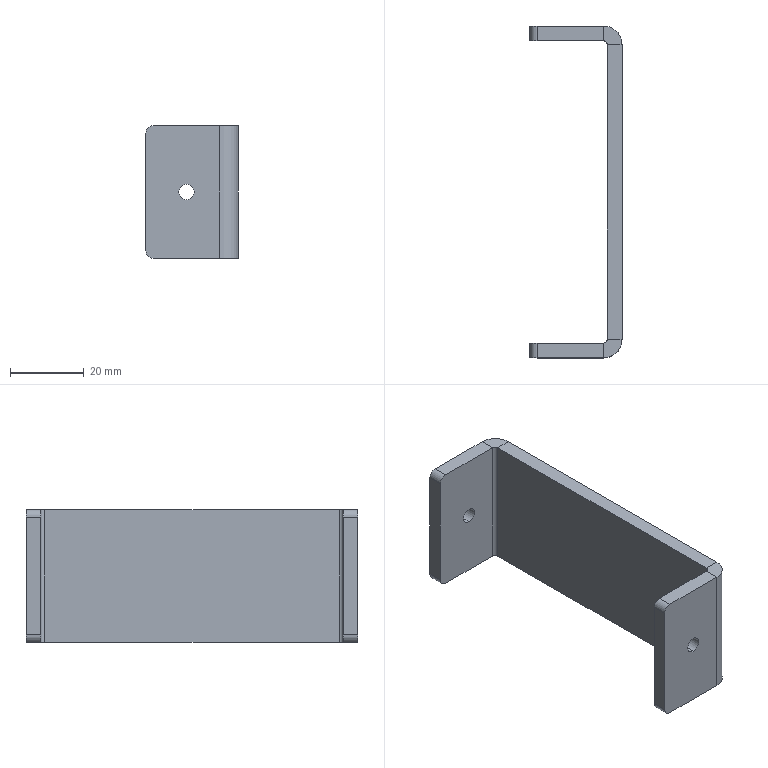Part | STEP file | Cang dai 2 | 1 solid | 30 faces | box 25 x 90 x 36 mm | volume 18513 mm3 | plane 18 | cylinder 12 | commonest cylinder face diameters 4 x4 4.2 x4 2 x2 10 x2
STEP:
#1=CARTESIAN_POINT('',(-14.,-41.,-2.1));
#2=VERTEX_POINT('',#1);
#3=CARTESIAN_POINT('',(-14.,-41.,2.1));
#4=VERTEX_POINT('',#3);
#5=CARTESIAN_POINT('',(-14.,-41.,0.));
#6=DIRECTION('',(0.,1.,0.));
#7=DIRECTION('',(0.,0.,1.));
#8=AXIS2_PLACEMENT_3D('',#5,#6,#7);
#9=CIRCLE('',#8,2.1);
#10=EDGE_CURVE('',#2,#4,#9,.T.);
#11=ORIENTED_EDGE('',*,*,#10,.T.);
#12=CARTESIAN_POINT('',(-14.,-45.,2.1));
#13=VERTEX_POINT('',#12);
#14=CARTESIAN_POINT('',(-14.,-45.,2.1));
#15=DIRECTION('',(0.,-1.,0.));
#16=VECTOR('',#15,1000.);
#17=LINE('',#14,#16);
#18=EDGE_CURVE('',#4,#13,#17,.T.);
#19=ORIENTED_EDGE('',*,*,#18,.T.);
#20=CARTESIAN_POINT('',(-14.,-45.,-2.1));
#21=VERTEX_POINT('',#20);
#22=CARTESIAN_POINT('',(-14.,-45.,0.));
#23=DIRECTION('',(0.,-1.,0.));
#24=DIRECTION('',(0.,0.,-1.));
#25=AXIS2_PLACEMENT_3D('',#22,#23,#24);
#26=CIRCLE('',#25,2.1);
#27=EDGE_CURVE('',#13,#21,#26,.T.);
#28=ORIENTED_EDGE('',*,*,#27,.T.);
#29=CARTESIAN_POINT('',(-14.,-45.,-2.1));
#30=DIRECTION('',(0.,-1.,0.));
#31=VECTOR('',#30,1000.);
#32=LINE('',#29,#31);
#33=EDGE_CURVE('',#2,#21,#32,.T.);
#34=ORIENTED_EDGE('',*,*,#33,.F.);
#35=EDGE_LOOP('',(#11,#19,#28,#34));
#36=FACE_OUTER_BOUND('',#35,.T.);
#37=CARTESIAN_POINT('',(-14.,-45.,0.));
#38=DIRECTION('',(0.,-1.,0.));
#39=DIRECTION('',(0.,0.,-1.));
#40=AXIS2_PLACEMENT_3D('',#37,#38,#39);
#41=CYLINDRICAL_SURFACE('',#40,2.1);
#42=ADVANCED_FACE('',(#36),#41,.F.);
#43=CARTESIAN_POINT('',(-14.,41.,2.1));
#44=VERTEX_POINT('',#43);
#45=CARTESIAN_POINT('',(-14.,41.,-2.1));
#46=VERTEX_POINT('',#45);
#47=CARTESIAN_POINT('',(-14.,41.,0.));
#48=DIRECTION('',(0.,-1.,0.));
#49=DIRECTION('',(0.,0.,-1.));
#50=AXIS2_PLACEMENT_3D('',#47,#48,#49);
#51=CIRCLE('',#50,2.1);
#52=EDGE_CURVE('',#44,#46,#51,.T.);
#53=ORIENTED_EDGE('',*,*,#52,.T.);
#54=CARTESIAN_POINT('',(-14.,45.,-2.1));
#55=VERTEX_POINT('',#54);
#56=CARTESIAN_POINT('',(-14.,45.,-2.1));
#57=DIRECTION('',(0.,1.,0.));
#58=VECTOR('',#57,1000.);
#59=LINE('',#56,#58);
#60=EDGE_CURVE('',#46,#55,#59,.T.);
#61=ORIENTED_EDGE('',*,*,#60,.T.);
#62=CARTESIAN_POINT('',(-14.,45.,2.1));
#63=VERTEX_POINT('',#62);
#64=CARTESIAN_POINT('',(-14.,45.,0.));
#65=DIRECTION('',(0.,1.,0.));
#66=DIRECTION('',(0.,0.,1.));
#67=AXIS2_PLACEMENT_3D('',#64,#65,#66);
#68=CIRCLE('',#67,2.1);
#69=EDGE_CURVE('',#55,#63,#68,.T.);
#70=ORIENTED_EDGE('',*,*,#69,.T.);
#71=CARTESIAN_POINT('',(-14.,45.,2.1));
#72=DIRECTION('',(0.,1.,0.));
#73=VECTOR('',#72,1000.);
#74=LINE('',#71,#73);
#75=EDGE_CURVE('',#44,#63,#74,.T.);
#76=ORIENTED_EDGE('',*,*,#75,.F.);
#77=EDGE_LOOP('',(#53,#61,#70,#76));
#78=FACE_OUTER_BOUND('',#77,.T.);
#79=CARTESIAN_POINT('',(-14.,45.,0.));
#80=DIRECTION('',(0.,1.,0.));
#81=DIRECTION('',(0.,0.,1.));
#82=AXIS2_PLACEMENT_3D('',#79,#80,#81);
#83=CYLINDRICAL_SURFACE('',#82,2.1);
#84=ADVANCED_FACE('',(#78),#83,.F.);
#85=CARTESIAN_POINT('',(-25.,-45.,16.));
#86=VERTEX_POINT('',#85);
#87=CARTESIAN_POINT('',(-25.,-45.,-16.));
#88=VERTEX_POINT('',#87);
#89=CARTESIAN_POINT('',(-25.,-45.,18.));
#90=DIRECTION('',(0.,0.,-1.));
#91=VECTOR('',#90,1000.);
#92=LINE('',#89,#91);
#93=EDGE_CURVE('',#86,#88,#92,.T.);
#94=ORIENTED_EDGE('',*,*,#93,.T.);
#95=CARTESIAN_POINT('',(-23.,-45.,-18.));
#96=VERTEX_POINT('',#95);
#97=CARTESIAN_POINT('',(-23.,-45.,-16.));
#98=DIRECTION('',(0.,-1.,0.));
#99=DIRECTION('',(0.,0.,1.));
#100=AXIS2_PLACEMENT_3D('',#97,#98,#99);
#101=CIRCLE('',#100,2.);
#102=EDGE_CURVE('',#88,#96,#101,.T.);
#103=ORIENTED_EDGE('',*,*,#102,.T.);
#104=CARTESIAN_POINT('',(-5.,-45.,-18.));
#105=VERTEX_POINT('',#104);
#106=CARTESIAN_POINT('',(0.,-45.,-18.));
#107=DIRECTION('',(1.,0.,0.));
#108=VECTOR('',#107,1000.);
#109=LINE('',#106,#108);
#110=EDGE_CURVE('',#96,#105,#109,.T.);
#111=ORIENTED_EDGE('',*,*,#110,.T.);
#112=CARTESIAN_POINT('',(-5.,-45.,18.));
#113=VERTEX_POINT('',#112);
#114=CARTESIAN_POINT('',(-5.,-45.,18.));
#115=DIRECTION('',(0.,0.,-1.));
#116=VECTOR('',#115,1000.);
#117=LINE('',#114,#116);
#118=EDGE_CURVE('',#113,#105,#117,.T.);
#119=ORIENTED_EDGE('',*,*,#118,.F.);
#120=CARTESIAN_POINT('',(-23.,-45.,18.));
#121=VERTEX_POINT('',#120);
#122=CARTESIAN_POINT('',(0.,-45.,18.));
#123=DIRECTION('',(1.,0.,0.));
#124=VECTOR('',#123,1000.);
#125=LINE('',#122,#124);
#126=EDGE_CURVE('',#121,#113,#125,.T.);
#127=ORIENTED_EDGE('',*,*,#126,.F.);
#128=CARTESIAN_POINT('',(-23.,-45.,16.));
#129=DIRECTION('',(0.,-1.,0.));
#130=DIRECTION('',(0.,0.,1.));
#131=AXIS2_PLACEMENT_3D('',#128,#129,#130);
#132=CIRCLE('',#131,2.);
#133=EDGE_CURVE('',#121,#86,#132,.T.);
#134=ORIENTED_EDGE('',*,*,#133,.T.);
#135=EDGE_LOOP('',(#94,#103,#111,#119,#127,#134));
#136=FACE_OUTER_BOUND('',#135,.T.);
#137=CARTESIAN_POINT('',(-14.,-45.,0.));
#138=DIRECTION('',(0.,-1.,0.));
#139=DIRECTION('',(0.,0.,-1.));
#140=AXIS2_PLACEMENT_3D('',#137,#138,#139);
#141=CIRCLE('',#140,2.1);
#142=EDGE_CURVE('',#21,#13,#141,.T.);
#143=ORIENTED_EDGE('',*,*,#142,.F.);
#144=ORIENTED_EDGE('',*,*,#27,.F.);
#145=EDGE_LOOP('',(#143,#144));
#146=FACE_BOUND('',#145,.T.);
#147=CARTESIAN_POINT('',(0.,-45.,18.));
#148=DIRECTION('',(0.,1.,0.));
#149=DIRECTION('',(0.,0.,1.));
#150=AXIS2_PLACEMENT_3D('',#147,#148,#149);
#151=PLANE('',#150);
#152=ADVANCED_FACE('',(#136,#146),#151,.F.);
#153=CARTESIAN_POINT('',(-5.,45.,-18.));
#154=VERTEX_POINT('',#153);
#155=CARTESIAN_POINT('',(-23.,45.,-18.));
#156=VERTEX_POINT('',#155);
#157=CARTESIAN_POINT('',(0.,45.,-18.));
#158=DIRECTION('',(-1.,0.,0.));
#159=VECTOR('',#158,1000.);
#160=LINE('',#157,#159);
#161=EDGE_CURVE('',#154,#156,#160,.T.);
#162=ORIENTED_EDGE('',*,*,#161,.T.);
#163=CARTESIAN_POINT('',(-25.,45.,-16.));
#164=VERTEX_POINT('',#163);
#165=CARTESIAN_POINT('',(-23.,45.,-16.));
#166=DIRECTION('',(0.,1.,0.));
#167=DIRECTION('',(0.,0.,-1.));
#168=AXIS2_PLACEMENT_3D('',#165,#166,#167);
#169=CIRCLE('',#168,2.);
#170=EDGE_CURVE('',#156,#164,#169,.T.);
#171=ORIENTED_EDGE('',*,*,#170,.T.);
#172=CARTESIAN_POINT('',(-25.,45.,16.));
#173=VERTEX_POINT('',#172);
#174=CARTESIAN_POINT('',(-25.,45.,18.));
#175=DIRECTION('',(0.,0.,-1.));
#176=VECTOR('',#175,1000.);
#177=LINE('',#174,#176);
#178=EDGE_CURVE('',#173,#164,#177,.T.);
#179=ORIENTED_EDGE('',*,*,#178,.F.);
#180=CARTESIAN_POINT('',(-23.,45.,18.));
#181=VERTEX_POINT('',#180);
#182=CARTESIAN_POINT('',(-23.,45.,16.));
#183=DIRECTION('',(0.,1.,0.));
#184=DIRECTION('',(0.,0.,-1.));
#185=AXIS2_PLACEMENT_3D('',#182,#183,#184);
#186=CIRCLE('',#185,2.);
#187=EDGE_CURVE('',#173,#181,#186,.T.);
#188=ORIENTED_EDGE('',*,*,#187,.T.);
#189=CARTESIAN_POINT('',(-5.,45.,18.));
#190=VERTEX_POINT('',#189);
#191=CARTESIAN_POINT('',(0.,45.,18.));
#192=DIRECTION('',(-1.,0.,0.));
#193=VECTOR('',#192,1000.);
#194=LINE('',#191,#193);
#195=EDGE_CURVE('',#190,#181,#194,.T.);
#196=ORIENTED_EDGE('',*,*,#195,.F.);
#197=CARTESIAN_POINT('',(-5.,45.,18.));
#198=DIRECTION('',(0.,0.,-1.));
#199=VECTOR('',#198,1000.);
#200=LINE('',#197,#199);
#201=EDGE_CURVE('',#190,#154,#200,.T.);
#202=ORIENTED_EDGE('',*,*,#201,.T.);
#203=EDGE_LOOP('',(#162,#171,#179,#188,#196,#202));
#204=FACE_OUTER_BOUND('',#203,.T.);
#205=CARTESIAN_POINT('',(-14.,45.,0.));
#206=DIRECTION('',(0.,1.,0.));
#207=DIRECTION('',(0.,0.,1.));
#208=AXIS2_PLACEMENT_3D('',#205,#206,#207);
#209=CIRCLE('',#208,2.1);
#210=EDGE_CURVE('',#63,#55,#209,.T.);
#211=ORIENTED_EDGE('',*,*,#210,.F.);
#212=ORIENTED_EDGE('',*,*,#69,.F.);
#213=EDGE_LOOP('',(#211,#212));
#214=FACE_BOUND('',#213,.T.);
#215=CARTESIAN_POINT('',(0.,45.,18.));
#216=DIRECTION('',(0.,-1.,0.));
#217=DIRECTION('',(0.,0.,-1.));
#218=AXIS2_PLACEMENT_3D('',#215,#216,#217);
#219=PLANE('',#218);
#220=ADVANCED_FACE('',(#204,#214),#219,.F.);
#221=CARTESIAN_POINT('',(-5.,-41.,18.));
#222=VERTEX_POINT('',#221);
#223=CARTESIAN_POINT('',(-5.,-45.,18.));
#224=DIRECTION('',(0.,1.,0.));
#225=VECTOR('',#224,1000.);
#226=LINE('',#223,#225);
#227=EDGE_CURVE('',#113,#222,#226,.T.);
#228=ORIENTED_EDGE('',*,*,#227,.F.);
#229=CARTESIAN_POINT('',(0.,-40.,18.));
#230=VERTEX_POINT('',#229);
#231=CARTESIAN_POINT('',(-5.,-40.,18.));
#232=DIRECTION('',(0.,0.,1.));
#233=DIRECTION('',(-1.,0.,0.));
#234=AXIS2_PLACEMENT_3D('',#231,#232,#233);
#235=CIRCLE('',#234,5.);
#236=EDGE_CURVE('',#113,#230,#235,.T.);
#237=ORIENTED_EDGE('',*,*,#236,.T.);
#238=CARTESIAN_POINT('',(-4.,-40.,18.));
#239=VERTEX_POINT('',#238);
#240=CARTESIAN_POINT('',(-4.,-40.,18.));
#241=DIRECTION('',(1.,0.,0.));
#242=VECTOR('',#241,1000.);
#243=LINE('',#240,#242);
#244=EDGE_CURVE('',#239,#230,#243,.T.);
#245=ORIENTED_EDGE('',*,*,#244,.F.);
#246=CARTESIAN_POINT('',(-5.,-40.,18.));
#247=DIRECTION('',(0.,0.,1.));
#248=DIRECTION('',(1.,0.,0.));
#249=AXIS2_PLACEMENT_3D('',#246,#247,#248);
#250=CIRCLE('',#249,1.);
#251=EDGE_CURVE('',#222,#239,#250,.T.);
#252=ORIENTED_EDGE('',*,*,#251,.F.);
#253=EDGE_LOOP('',(#228,#237,#245,#252));
#254=FACE_OUTER_BOUND('',#253,.T.);
#255=CARTESIAN_POINT('',(-5.,-45.,18.));
#256=DIRECTION('',(0.,0.,1.));
#257=DIRECTION('',(1.,0.,0.));
#258=AXIS2_PLACEMENT_3D('',#255,#256,#257);
#259=PLANE('',#258);
#260=ADVANCED_FACE('',(#254),#259,.T.);
#261=CARTESIAN_POINT('',(-23.,-41.,18.));
#262=VERTEX_POINT('',#261);
#263=CARTESIAN_POINT('',(0.,-41.,18.));
#264=DIRECTION('',(1.,0.,0.));
#265=VECTOR('',#264,1000.);
#266=LINE('',#263,#265);
#267=EDGE_CURVE('',#262,#222,#266,.T.);
#268=ORIENTED_EDGE('',*,*,#267,.F.);
#269=CARTESIAN_POINT('',(-23.,-40.,18.));
#270=DIRECTION('',(0.,-1.,0.));
#271=VECTOR('',#270,1000.);
#272=LINE('',#269,#271);
#273=EDGE_CURVE('',#262,#121,#272,.T.);
#274=ORIENTED_EDGE('',*,*,#273,.T.);
#275=ORIENTED_EDGE('',*,*,#126,.T.);
#276=ORIENTED_EDGE('',*,*,#227,.T.);
#277=EDGE_LOOP('',(#268,#274,#275,#276));
#278=FACE_OUTER_BOUND('',#277,.T.);
#279=CARTESIAN_POINT('',(-4.,-40.,18.));
#280=DIRECTION('',(0.,0.,1.));
#281=DIRECTION('',(1.,0.,0.));
#282=AXIS2_PLACEMENT_3D('',#279,#280,#281);
#283=PLANE('',#282);
#284=ADVANCED_FACE('',(#278),#283,.T.);
#285=CARTESIAN_POINT('',(0.,-40.,-18.));
#286=VERTEX_POINT('',#285);
#287=CARTESIAN_POINT('',(-4.,-40.,-18.));
#288=VERTEX_POINT('',#287);
#289=CARTESIAN_POINT('',(0.,-40.,-18.));
#290=DIRECTION('',(-1.,0.,0.));
#291=VECTOR('',#290,1000.);
#292=LINE('',#289,#291);
#293=EDGE_CURVE('',#286,#288,#292,.T.);
#294=ORIENTED_EDGE('',*,*,#293,.F.);
#295=CARTESIAN_POINT('',(-5.,-40.,-18.));
#296=DIRECTION('',(0.,0.,1.));
#297=DIRECTION('',(-1.,0.,0.));
#298=AXIS2_PLACEMENT_3D('',#295,#296,#297);
#299=CIRCLE('',#298,5.);
#300=EDGE_CURVE('',#105,#286,#299,.T.);
#301=ORIENTED_EDGE('',*,*,#300,.F.);
#302=CARTESIAN_POINT('',(-5.,-41.,-18.));
#303=VERTEX_POINT('',#302);
#304=CARTESIAN_POINT('',(-5.,-41.,-18.));
#305=DIRECTION('',(0.,-1.,0.));
#306=VECTOR('',#305,1000.);
#307=LINE('',#304,#306);
#308=EDGE_CURVE('',#303,#105,#307,.T.);
#309=ORIENTED_EDGE('',*,*,#308,.F.);
#310=CARTESIAN_POINT('',(-5.,-40.,-18.));
#311=DIRECTION('',(0.,0.,1.));
#312=DIRECTION('',(1.,0.,0.));
#313=AXIS2_PLACEMENT_3D('',#310,#311,#312);
#314=CIRCLE('',#313,1.);
#315=EDGE_CURVE('',#303,#288,#314,.T.);
#316=ORIENTED_EDGE('',*,*,#315,.T.);
#317=EDGE_LOOP('',(#294,#301,#309,#316));
#318=FACE_OUTER_BOUND('',#317,.T.);
#319=CARTESIAN_POINT('',(0.,-40.,-18.));
#320=DIRECTION('',(0.,0.,-1.));
#321=DIRECTION('',(-1.,0.,0.));
#322=AXIS2_PLACEMENT_3D('',#319,#320,#321);
#323=PLANE('',#322);
#324=ADVANCED_FACE('',(#318),#323,.T.);
#325=CARTESIAN_POINT('',(0.,40.,-18.));
#326=VERTEX_POINT('',#325);
#327=CARTESIAN_POINT('',(0.,45.,-18.));
#328=DIRECTION('',(0.,1.,0.));
#329=VECTOR('',#328,1000.);
#330=LINE('',#327,#329);
#331=EDGE_CURVE('',#286,#326,#330,.T.);
#332=ORIENTED_EDGE('',*,*,#331,.F.);
#333=ORIENTED_EDGE('',*,*,#293,.T.);
#334=CARTESIAN_POINT('',(-4.,40.,-18.));
#335=VERTEX_POINT('',#334);
#336=CARTESIAN_POINT('',(-4.,45.,-18.));
#337=DIRECTION('',(0.,1.,0.));
#338=VECTOR('',#337,1000.);
#339=LINE('',#336,#338);
#340=EDGE_CURVE('',#288,#335,#339,.T.);
#341=ORIENTED_EDGE('',*,*,#340,.T.);
#342=CARTESIAN_POINT('',(-4.,40.,-18.));
#343=DIRECTION('',(1.,0.,0.));
#344=VECTOR('',#343,1000.);
#345=LINE('',#342,#344);
#346=EDGE_CURVE('',#335,#326,#345,.T.);
#347=ORIENTED_EDGE('',*,*,#346,.T.);
#348=EDGE_LOOP('',(#332,#333,#341,#347));
#349=FACE_OUTER_BOUND('',#348,.T.);
#350=CARTESIAN_POINT('',(-5.,-41.,-18.));
#351=DIRECTION('',(0.,0.,-1.));
#352=DIRECTION('',(-1.,0.,0.));
#353=AXIS2_PLACEMENT_3D('',#350,#351,#352);
#354=PLANE('',#353);
#355=ADVANCED_FACE('',(#349),#354,.T.);
#356=CARTESIAN_POINT('',(0.,40.,18.));
#357=VERTEX_POINT('',#356);
#358=CARTESIAN_POINT('',(-4.,40.,18.));
#359=VERTEX_POINT('',#358);
#360=CARTESIAN_POINT('',(0.,40.,18.));
#361=DIRECTION('',(-1.,0.,0.));
#362=VECTOR('',#361,1000.);
#363=LINE('',#360,#362);
#364=EDGE_CURVE('',#357,#359,#363,.T.);
#365=ORIENTED_EDGE('',*,*,#364,.F.);
#366=CARTESIAN_POINT('',(-5.,40.,18.));
#367=DIRECTION('',(0.,0.,1.));
#368=DIRECTION('',(-1.,0.,0.));
#369=AXIS2_PLACEMENT_3D('',#366,#367,#368);
#370=CIRCLE('',#369,5.);
#371=EDGE_CURVE('',#357,#190,#370,.T.);
#372=ORIENTED_EDGE('',*,*,#371,.T.);
#373=CARTESIAN_POINT('',(-5.,41.,18.));
#374=VERTEX_POINT('',#373);
#375=CARTESIAN_POINT('',(-5.,41.,18.));
#376=DIRECTION('',(0.,1.,0.));
#377=VECTOR('',#376,1000.);
#378=LINE('',#375,#377);
#379=EDGE_CURVE('',#374,#190,#378,.T.);
#380=ORIENTED_EDGE('',*,*,#379,.F.);
#381=CARTESIAN_POINT('',(-5.,40.,18.));
#382=DIRECTION('',(0.,0.,1.));
#383=DIRECTION('',(1.,0.,0.));
#384=AXIS2_PLACEMENT_3D('',#381,#382,#383);
#385=CIRCLE('',#384,1.);
#386=EDGE_CURVE('',#359,#374,#385,.T.);
#387=ORIENTED_EDGE('',*,*,#386,.F.);
#388=EDGE_LOOP('',(#365,#372,#380,#387));
#389=FACE_OUTER_BOUND('',#388,.T.);
#390=CARTESIAN_POINT('',(0.,40.,18.));
#391=DIRECTION('',(0.,0.,1.));
#392=DIRECTION('',(1.,0.,0.));
#393=AXIS2_PLACEMENT_3D('',#390,#391,#392);
#394=PLANE('',#393);
#395=ADVANCED_FACE('',(#389),#394,.T.);
#396=CARTESIAN_POINT('',(0.,45.,18.));
#397=DIRECTION('',(0.,1.,0.));
#398=VECTOR('',#397,1000.);
#399=LINE('',#396,#398);
#400=EDGE_CURVE('',#230,#357,#399,.T.);
#401=ORIENTED_EDGE('',*,*,#400,.T.);
#402=ORIENTED_EDGE('',*,*,#364,.T.);
#403=CARTESIAN_POINT('',(-4.,45.,18.));
#404=DIRECTION('',(0.,1.,0.));
#405=VECTOR('',#404,1000.);
#406=LINE('',#403,#405);
#407=EDGE_CURVE('',#239,#359,#406,.T.);
#408=ORIENTED_EDGE('',*,*,#407,.F.);
#409=ORIENTED_EDGE('',*,*,#244,.T.);
#410=EDGE_LOOP('',(#401,#402,#408,#409));
#411=FACE_OUTER_BOUND('',#410,.T.);
#412=CARTESIAN_POINT('',(-5.,41.,18.));
#413=DIRECTION('',(0.,0.,1.));
#414=DIRECTION('',(1.,0.,0.));
#415=AXIS2_PLACEMENT_3D('',#412,#413,#414);
#416=PLANE('',#415);
#417=ADVANCED_FACE('',(#411),#416,.T.);
#418=CARTESIAN_POINT('',(-5.,41.,-18.));
#419=VERTEX_POINT('',#418);
#420=CARTESIAN_POINT('',(-5.,45.,-18.));
#421=DIRECTION('',(0.,-1.,0.));
#422=VECTOR('',#421,1000.);
#423=LINE('',#420,#422);
#424=EDGE_CURVE('',#154,#419,#423,.T.);
#425=ORIENTED_EDGE('',*,*,#424,.F.);
#426=CARTESIAN_POINT('',(-5.,40.,-18.));
#427=DIRECTION('',(0.,0.,1.));
#428=DIRECTION('',(-1.,0.,0.));
#429=AXIS2_PLACEMENT_3D('',#426,#427,#428);
#430=CIRCLE('',#429,5.);
#431=EDGE_CURVE('',#326,#154,#430,.T.);
#432=ORIENTED_EDGE('',*,*,#431,.F.);
#433=ORIENTED_EDGE('',*,*,#346,.F.);
#434=CARTESIAN_POINT('',(-5.,40.,-18.));
#435=DIRECTION('',(0.,0.,1.));
#436=DIRECTION('',(1.,0.,0.));
#437=AXIS2_PLACEMENT_3D('',#434,#435,#436);
#438=CIRCLE('',#437,1.);
#439=EDGE_CURVE('',#335,#419,#438,.T.);
#440=ORIENTED_EDGE('',*,*,#439,.T.);
#441=EDGE_LOOP('',(#425,#432,#433,#440));
#442=FACE_OUTER_BOUND('',#441,.T.);
#443=CARTESIAN_POINT('',(-5.,45.,-18.));
#444=DIRECTION('',(0.,0.,-1.));
#445=DIRECTION('',(-1.,0.,0.));
#446=AXIS2_PLACEMENT_3D('',#443,#444,#445);
#447=PLANE('',#446);
#448=ADVANCED_FACE('',(#442),#447,.T.);
#449=CARTESIAN_POINT('',(-23.,41.,-18.));
#450=VERTEX_POINT('',#449);
#451=CARTESIAN_POINT('',(0.,41.,-18.));
#452=DIRECTION('',(-1.,0.,0.));
#453=VECTOR('',#452,1000.);
#454=LINE('',#451,#453);
#455=EDGE_CURVE('',#419,#450,#454,.T.);
#456=ORIENTED_EDGE('',*,*,#455,.T.);
#457=CARTESIAN_POINT('',(-23.,40.,-18.));
#458=DIRECTION('',(0.,1.,0.));
#459=VECTOR('',#458,1000.);
#460=LINE('',#457,#459);
#461=EDGE_CURVE('',#450,#156,#460,.T.);
#462=ORIENTED_EDGE('',*,*,#461,.T.);
#463=ORIENTED_EDGE('',*,*,#161,.F.);
#464=ORIENTED_EDGE('',*,*,#424,.T.);
#465=EDGE_LOOP('',(#456,#462,#463,#464));
#466=FACE_OUTER_BOUND('',#465,.T.);
#467=CARTESIAN_POINT('',(-4.,40.,-18.));
#468=DIRECTION('',(0.,0.,-1.));
#469=DIRECTION('',(-1.,0.,0.));
#470=AXIS2_PLACEMENT_3D('',#467,#468,#469);
#471=PLANE('',#470);
#472=ADVANCED_FACE('',(#466),#471,.T.);
#473=ORIENTED_EDGE('',*,*,#178,.T.);
#474=CARTESIAN_POINT('',(-25.,41.,-16.));
#475=VERTEX_POINT('',#474);
#476=CARTESIAN_POINT('',(-25.,41.,-16.));
#477=DIRECTION('',(0.,-1.,0.));
#478=VECTOR('',#477,1000.);
#479=LINE('',#476,#478);
#480=EDGE_CURVE('',#164,#475,#479,.T.);
#481=ORIENTED_EDGE('',*,*,#480,.T.);
#482=CARTESIAN_POINT('',(-25.,41.,16.));
#483=VERTEX_POINT('',#482);
#484=CARTESIAN_POINT('',(-25.,41.,18.));
#485=DIRECTION('',(0.,0.,-1.));
#486=VECTOR('',#485,1000.);
#487=LINE('',#484,#486);
#488=EDGE_CURVE('',#483,#475,#487,.T.);
#489=ORIENTED_EDGE('',*,*,#488,.F.);
#490=CARTESIAN_POINT('',(-25.,41.,16.));
#491=DIRECTION('',(0.,1.,0.));
#492=VECTOR('',#491,1000.);
#493=LINE('',#490,#492);
#494=EDGE_CURVE('',#483,#173,#493,.T.);
#495=ORIENTED_EDGE('',*,*,#494,.T.);
#496=EDGE_LOOP('',(#473,#481,#489,#495));
#497=FACE_OUTER_BOUND('',#496,.T.);
#498=CARTESIAN_POINT('',(-25.,41.,18.));
#499=DIRECTION('',(-1.,0.,0.));
#500=DIRECTION('',(0.,0.,1.));
#501=AXIS2_PLACEMENT_3D('',#498,#499,#500);
#502=PLANE('',#501);
#503=ADVANCED_FACE('',(#497),#502,.T.);
#504=ORIENTED_EDGE('',*,*,#52,.F.);
#505=CARTESIAN_POINT('',(-14.,41.,0.));
#506=DIRECTION('',(0.,-1.,0.));
#507=DIRECTION('',(0.,0.,-1.));
#508=AXIS2_PLACEMENT_3D('',#505,#506,#507);
#509=CIRCLE('',#508,2.1);
#510=EDGE_CURVE('',#46,#44,#509,.T.);
#511=ORIENTED_EDGE('',*,*,#510,.F.);
#512=EDGE_LOOP('',(#504,#511));
#513=FACE_BOUND('',#512,.T.);
#514=ORIENTED_EDGE('',*,*,#488,.T.);
#515=CARTESIAN_POINT('',(-23.,41.,-16.));
#516=DIRECTION('',(0.,-1.,0.));
#517=DIRECTION('',(0.,0.,-1.));
#518=AXIS2_PLACEMENT_3D('',#515,#516,#517);
#519=CIRCLE('',#518,2.);
#520=EDGE_CURVE('',#475,#450,#519,.T.);
#521=ORIENTED_EDGE('',*,*,#520,.T.);
#522=ORIENTED_EDGE('',*,*,#455,.F.);
#523=CARTESIAN_POINT('',(-5.,41.,18.));
#524=DIRECTION('',(0.,0.,-1.));
#525=VECTOR('',#524,1000.);
#526=LINE('',#523,#525);
#527=EDGE_CURVE('',#374,#419,#526,.T.);
#528=ORIENTED_EDGE('',*,*,#527,.F.);
#529=CARTESIAN_POINT('',(-23.,41.,18.));
#530=VERTEX_POINT('',#529);
#531=CARTESIAN_POINT('',(0.,41.,18.));
#532=DIRECTION('',(-1.,0.,0.));
#533=VECTOR('',#532,1000.);
#534=LINE('',#531,#533);
#535=EDGE_CURVE('',#374,#530,#534,.T.);
#536=ORIENTED_EDGE('',*,*,#535,.T.);
#537=CARTESIAN_POINT('',(-23.,41.,16.));
#538=DIRECTION('',(0.,-1.,0.));
#539=DIRECTION('',(0.,0.,-1.));
#540=AXIS2_PLACEMENT_3D('',#537,#538,#539);
#541=CIRCLE('',#540,2.);
#542=EDGE_CURVE('',#530,#483,#541,.T.);
#543=ORIENTED_EDGE('',*,*,#542,.T.);
#544=EDGE_LOOP('',(#514,#521,#522,#528,#536,#543));
#545=FACE_OUTER_BOUND('',#544,.T.);
#546=CARTESIAN_POINT('',(0.,41.,18.));
#547=DIRECTION('',(0.,-1.,0.));
#548=DIRECTION('',(0.,0.,-1.));
#549=AXIS2_PLACEMENT_3D('',#546,#547,#548);
#550=PLANE('',#549);
#551=ADVANCED_FACE('',(#513,#545),#550,.T.);
#552=ORIENTED_EDGE('',*,*,#439,.F.);
#553=CARTESIAN_POINT('',(-4.,40.,18.));
#554=DIRECTION('',(0.,0.,-1.));
#555=VECTOR('',#554,1000.);
#556=LINE('',#553,#555);
#557=EDGE_CURVE('',#359,#335,#556,.T.);
#558=ORIENTED_EDGE('',*,*,#557,.F.);
#559=ORIENTED_EDGE('',*,*,#386,.T.);
#560=ORIENTED_EDGE('',*,*,#527,.T.);
#561=EDGE_LOOP('',(#552,#558,#559,#560));
#562=FACE_OUTER_BOUND('',#561,.T.);
#563=CARTESIAN_POINT('',(-5.,40.,18.));
#564=DIRECTION('',(0.,0.,-1.));
#565=DIRECTION('',(-1.,0.,0.));
#566=AXIS2_PLACEMENT_3D('',#563,#564,#565);
#567=CYLINDRICAL_SURFACE('',#566,1.);
#568=ADVANCED_FACE('',(#562),#567,.F.);
#569=ORIENTED_EDGE('',*,*,#340,.F.);
#570=CARTESIAN_POINT('',(-4.,-40.,18.));
#571=DIRECTION('',(0.,0.,-1.));
#572=VECTOR('',#571,1000.);
#573=LINE('',#570,#572);
#574=EDGE_CURVE('',#239,#288,#573,.T.);
#575=ORIENTED_EDGE('',*,*,#574,.F.);
#576=ORIENTED_EDGE('',*,*,#407,.T.);
#577=ORIENTED_EDGE('',*,*,#557,.T.);
#578=EDGE_LOOP('',(#569,#575,#576,#577));
#579=FACE_OUTER_BOUND('',#578,.T.);
#580=CARTESIAN_POINT('',(-4.,45.,18.));
#581=DIRECTION('',(-1.,0.,0.));
#582=DIRECTION('',(0.,0.,1.));
#583=AXIS2_PLACEMENT_3D('',#580,#581,#582);
#584=PLANE('',#583);
#585=ADVANCED_FACE('',(#579),#584,.T.);
#586=ORIENTED_EDGE('',*,*,#315,.F.);
#587=CARTESIAN_POINT('',(-5.,-41.,18.));
#588=DIRECTION('',(0.,0.,-1.));
#589=VECTOR('',#588,1000.);
#590=LINE('',#587,#589);
#591=EDGE_CURVE('',#222,#303,#590,.T.);
#592=ORIENTED_EDGE('',*,*,#591,.F.);
#593=ORIENTED_EDGE('',*,*,#251,.T.);
#594=ORIENTED_EDGE('',*,*,#574,.T.);
#595=EDGE_LOOP('',(#586,#592,#593,#594));
#596=FACE_OUTER_BOUND('',#595,.T.);
#597=CARTESIAN_POINT('',(-5.,-40.,18.));
#598=DIRECTION('',(0.,0.,-1.));
#599=DIRECTION('',(-1.,0.,0.));
#600=AXIS2_PLACEMENT_3D('',#597,#598,#599);
#601=CYLINDRICAL_SURFACE('',#600,1.);
#602=ADVANCED_FACE('',(#596),#601,.F.);
#603=ORIENTED_EDGE('',*,*,#10,.F.);
#604=CARTESIAN_POINT('',(-14.,-41.,0.));
#605=DIRECTION('',(0.,1.,0.));
#606=DIRECTION('',(0.,0.,1.));
#607=AXIS2_PLACEMENT_3D('',#604,#605,#606);
#608=CIRCLE('',#607,2.1);
#609=EDGE_CURVE('',#4,#2,#608,.T.);
#610=ORIENTED_EDGE('',*,*,#609,.F.);
#611=EDGE_LOOP('',(#603,#610));
#612=FACE_BOUND('',#611,.T.);
#613=CARTESIAN_POINT('',(-23.,-41.,-18.));
#614=VERTEX_POINT('',#613);
#615=CARTESIAN_POINT('',(0.,-41.,-18.));
#616=DIRECTION('',(1.,0.,0.));
#617=VECTOR('',#616,1000.);
#618=LINE('',#615,#617);
#619=EDGE_CURVE('',#614,#303,#618,.T.);
#620=ORIENTED_EDGE('',*,*,#619,.F.);
#621=CARTESIAN_POINT('',(-25.,-41.,-16.));
#622=VERTEX_POINT('',#621);
#623=CARTESIAN_POINT('',(-23.,-41.,-16.));
#624=DIRECTION('',(0.,1.,0.));
#625=DIRECTION('',(0.,0.,1.));
#626=AXIS2_PLACEMENT_3D('',#623,#624,#625);
#627=CIRCLE('',#626,2.);
#628=EDGE_CURVE('',#614,#622,#627,.T.);
#629=ORIENTED_EDGE('',*,*,#628,.T.);
#630=CARTESIAN_POINT('',(-25.,-41.,16.));
#631=VERTEX_POINT('',#630);
#632=CARTESIAN_POINT('',(-25.,-41.,18.));
#633=DIRECTION('',(0.,0.,-1.));
#634=VECTOR('',#633,1000.);
#635=LINE('',#632,#634);
#636=EDGE_CURVE('',#631,#622,#635,.T.);
#637=ORIENTED_EDGE('',*,*,#636,.F.);
#638=CARTESIAN_POINT('',(-23.,-41.,16.));
#639=DIRECTION('',(0.,1.,0.));
#640=DIRECTION('',(0.,0.,1.));
#641=AXIS2_PLACEMENT_3D('',#638,#639,#640);
#642=CIRCLE('',#641,2.);
#643=EDGE_CURVE('',#631,#262,#642,.T.);
#644=ORIENTED_EDGE('',*,*,#643,.T.);
#645=ORIENTED_EDGE('',*,*,#267,.T.);
#646=ORIENTED_EDGE('',*,*,#591,.T.);
#647=EDGE_LOOP('',(#620,#629,#637,#644,#645,#646));
#648=FACE_OUTER_BOUND('',#647,.T.);
#649=CARTESIAN_POINT('',(0.,-41.,18.));
#650=DIRECTION('',(0.,1.,0.));
#651=DIRECTION('',(0.,0.,1.));
#652=AXIS2_PLACEMENT_3D('',#649,#650,#651);
#653=PLANE('',#652);
#654=ADVANCED_FACE('',(#612,#648),#653,.T.);
#655=ORIENTED_EDGE('',*,*,#636,.T.);
#656=CARTESIAN_POINT('',(-25.,-45.,-16.));
#657=DIRECTION('',(0.,-1.,0.));
#658=VECTOR('',#657,1000.);
#659=LINE('',#656,#658);
#660=EDGE_CURVE('',#622,#88,#659,.T.);
#661=ORIENTED_EDGE('',*,*,#660,.T.);
#662=ORIENTED_EDGE('',*,*,#93,.F.);
#663=CARTESIAN_POINT('',(-25.,-45.,16.));
#664=DIRECTION('',(0.,1.,0.));
#665=VECTOR('',#664,1000.);
#666=LINE('',#663,#665);
#667=EDGE_CURVE('',#86,#631,#666,.T.);
#668=ORIENTED_EDGE('',*,*,#667,.T.);
#669=EDGE_LOOP('',(#655,#661,#662,#668));
#670=FACE_OUTER_BOUND('',#669,.T.);
#671=CARTESIAN_POINT('',(-25.,-45.,18.));
#672=DIRECTION('',(-1.,0.,0.));
#673=DIRECTION('',(0.,0.,1.));
#674=AXIS2_PLACEMENT_3D('',#671,#672,#673);
#675=PLANE('',#674);
#676=ADVANCED_FACE('',(#670),#675,.T.);
#677=ORIENTED_EDGE('',*,*,#300,.T.);
#678=CARTESIAN_POINT('',(0.,-40.,18.));
#679=DIRECTION('',(0.,0.,-1.));
#680=VECTOR('',#679,1000.);
#681=LINE('',#678,#680);
#682=EDGE_CURVE('',#230,#286,#681,.T.);
#683=ORIENTED_EDGE('',*,*,#682,.F.);
#684=ORIENTED_EDGE('',*,*,#236,.F.);
#685=ORIENTED_EDGE('',*,*,#118,.T.);
#686=EDGE_LOOP('',(#677,#683,#684,#685));
#687=FACE_OUTER_BOUND('',#686,.T.);
#688=CARTESIAN_POINT('',(-5.,-40.,18.));
#689=DIRECTION('',(0.,0.,-1.));
#690=DIRECTION('',(-1.,0.,0.));
#691=AXIS2_PLACEMENT_3D('',#688,#689,#690);
#692=CYLINDRICAL_SURFACE('',#691,5.);
#693=ADVANCED_FACE('',(#687),#692,.T.);
#694=ORIENTED_EDGE('',*,*,#331,.T.);
#695=CARTESIAN_POINT('',(0.,40.,18.));
#696=DIRECTION('',(0.,0.,-1.));
#697=VECTOR('',#696,1000.);
#698=LINE('',#695,#697);
#699=EDGE_CURVE('',#357,#326,#698,.T.);
#700=ORIENTED_EDGE('',*,*,#699,.F.);
#701=ORIENTED_EDGE('',*,*,#400,.F.);
#702=ORIENTED_EDGE('',*,*,#682,.T.);
#703=EDGE_LOOP('',(#694,#700,#701,#702));
#704=FACE_OUTER_BOUND('',#703,.T.);
#705=CARTESIAN_POINT('',(0.,45.,18.));
#706=DIRECTION('',(-1.,0.,0.));
#707=DIRECTION('',(0.,0.,1.));
#708=AXIS2_PLACEMENT_3D('',#705,#706,#707);
#709=PLANE('',#708);
#710=ADVANCED_FACE('',(#704),#709,.F.);
#711=ORIENTED_EDGE('',*,*,#431,.T.);
#712=ORIENTED_EDGE('',*,*,#201,.F.);
#713=ORIENTED_EDGE('',*,*,#371,.F.);
#714=ORIENTED_EDGE('',*,*,#699,.T.);
#715=EDGE_LOOP('',(#711,#712,#713,#714));
#716=FACE_OUTER_BOUND('',#715,.T.);
#717=CARTESIAN_POINT('',(-5.,40.,18.));
#718=DIRECTION('',(0.,0.,-1.));
#719=DIRECTION('',(-1.,0.,0.));
#720=AXIS2_PLACEMENT_3D('',#717,#718,#719);
#721=CYLINDRICAL_SURFACE('',#720,5.);
#722=ADVANCED_FACE('',(#716),#721,.T.);
#723=ORIENTED_EDGE('',*,*,#195,.T.);
#724=CARTESIAN_POINT('',(-23.,40.,18.));
#725=DIRECTION('',(0.,-1.,0.));
#726=VECTOR('',#725,1000.);
#727=LINE('',#724,#726);
#728=EDGE_CURVE('',#181,#530,#727,.T.);
#729=ORIENTED_EDGE('',*,*,#728,.T.);
#730=ORIENTED_EDGE('',*,*,#535,.F.);
#731=ORIENTED_EDGE('',*,*,#379,.T.);
#732=EDGE_LOOP('',(#723,#729,#730,#731));
#733=FACE_OUTER_BOUND('',#732,.T.);
#734=CARTESIAN_POINT('',(-5.,40.,18.));
#735=DIRECTION('',(0.,0.,1.));
#736=DIRECTION('',(1.,0.,0.));
#737=AXIS2_PLACEMENT_3D('',#734,#735,#736);
#738=PLANE('',#737);
#739=ADVANCED_FACE('',(#733),#738,.T.);
#740=ORIENTED_EDGE('',*,*,#110,.F.);
#741=CARTESIAN_POINT('',(-23.,-41.,-18.));
#742=DIRECTION('',(0.,1.,0.));
#743=VECTOR('',#742,1000.);
#744=LINE('',#741,#743);
#745=EDGE_CURVE('',#96,#614,#744,.T.);
#746=ORIENTED_EDGE('',*,*,#745,.T.);
#747=ORIENTED_EDGE('',*,*,#619,.T.);
#748=ORIENTED_EDGE('',*,*,#308,.T.);
#749=EDGE_LOOP('',(#740,#746,#747,#748));
#750=FACE_OUTER_BOUND('',#749,.T.);
#751=CARTESIAN_POINT('',(-5.,40.,-18.));
#752=DIRECTION('',(0.,0.,1.));
#753=DIRECTION('',(1.,0.,0.));
#754=AXIS2_PLACEMENT_3D('',#751,#752,#753);
#755=PLANE('',#754);
#756=ADVANCED_FACE('',(#750),#755,.F.);
#757=ORIENTED_EDGE('',*,*,#102,.F.);
#758=ORIENTED_EDGE('',*,*,#660,.F.);
#759=ORIENTED_EDGE('',*,*,#628,.F.);
#760=ORIENTED_EDGE('',*,*,#745,.F.);
#761=EDGE_LOOP('',(#757,#758,#759,#760));
#762=FACE_OUTER_BOUND('',#761,.T.);
#763=CARTESIAN_POINT('',(-23.,40.,-16.));
#764=DIRECTION('',(0.,-1.,0.));
#765=DIRECTION('',(0.,0.,-1.));
#766=AXIS2_PLACEMENT_3D('',#763,#764,#765);
#767=CYLINDRICAL_SURFACE('',#766,2.);
#768=ADVANCED_FACE('',(#762),#767,.T.);
#769=ORIENTED_EDGE('',*,*,#133,.F.);
#770=ORIENTED_EDGE('',*,*,#273,.F.);
#771=ORIENTED_EDGE('',*,*,#643,.F.);
#772=ORIENTED_EDGE('',*,*,#667,.F.);
#773=EDGE_LOOP('',(#769,#770,#771,#772));
#774=FACE_OUTER_BOUND('',#773,.T.);
#775=CARTESIAN_POINT('',(-23.,-45.,16.));
#776=DIRECTION('',(0.,1.,0.));
#777=DIRECTION('',(0.,0.,1.));
#778=AXIS2_PLACEMENT_3D('',#775,#776,#777);
#779=CYLINDRICAL_SURFACE('',#778,2.);
#780=ADVANCED_FACE('',(#774),#779,.T.);
#781=ORIENTED_EDGE('',*,*,#520,.F.);
#782=ORIENTED_EDGE('',*,*,#480,.F.);
#783=ORIENTED_EDGE('',*,*,#170,.F.);
#784=ORIENTED_EDGE('',*,*,#461,.F.);
#785=EDGE_LOOP('',(#781,#782,#783,#784));
#786=FACE_OUTER_BOUND('',#785,.T.);
#787=CARTESIAN_POINT('',(-23.,40.,-16.));
#788=DIRECTION('',(0.,1.,0.));
#789=DIRECTION('',(0.,0.,1.));
#790=AXIS2_PLACEMENT_3D('',#787,#788,#789);
#791=CYLINDRICAL_SURFACE('',#790,2.);
#792=ADVANCED_FACE('',(#786),#791,.T.);
#793=ORIENTED_EDGE('',*,*,#542,.F.);
#794=ORIENTED_EDGE('',*,*,#728,.F.);
#795=ORIENTED_EDGE('',*,*,#187,.F.);
#796=ORIENTED_EDGE('',*,*,#494,.F.);
#797=EDGE_LOOP('',(#793,#794,#795,#796));
#798=FACE_OUTER_BOUND('',#797,.T.);
#799=CARTESIAN_POINT('',(-23.,41.,16.));
#800=DIRECTION('',(0.,1.,0.));
#801=DIRECTION('',(0.,0.,1.));
#802=AXIS2_PLACEMENT_3D('',#799,#800,#801);
#803=CYLINDRICAL_SURFACE('',#802,2.);
#804=ADVANCED_FACE('',(#798),#803,.T.);
#805=ORIENTED_EDGE('',*,*,#60,.F.);
#806=ORIENTED_EDGE('',*,*,#510,.T.);
#807=ORIENTED_EDGE('',*,*,#75,.T.);
#808=ORIENTED_EDGE('',*,*,#210,.T.);
#809=EDGE_LOOP('',(#805,#806,#807,#808));
#810=FACE_OUTER_BOUND('',#809,.T.);
#811=CARTESIAN_POINT('',(-14.,45.,0.));
#812=DIRECTION('',(0.,1.,0.));
#813=DIRECTION('',(0.,0.,1.));
#814=AXIS2_PLACEMENT_3D('',#811,#812,#813);
#815=CYLINDRICAL_SURFACE('',#814,2.1);
#816=ADVANCED_FACE('',(#810),#815,.F.);
#817=ORIENTED_EDGE('',*,*,#18,.F.);
#818=ORIENTED_EDGE('',*,*,#609,.T.);
#819=ORIENTED_EDGE('',*,*,#33,.T.);
#820=ORIENTED_EDGE('',*,*,#142,.T.);
#821=EDGE_LOOP('',(#817,#818,#819,#820));
#822=FACE_OUTER_BOUND('',#821,.T.);
#823=CARTESIAN_POINT('',(-14.,-45.,0.));
#824=DIRECTION('',(0.,-1.,0.));
#825=DIRECTION('',(0.,0.,-1.));
#826=AXIS2_PLACEMENT_3D('',#823,#824,#825);
#827=CYLINDRICAL_SURFACE('',#826,2.1);
#828=ADVANCED_FACE('',(#822),#827,.F.);
#829=CLOSED_SHELL('',(#42,#84,#152,#220,#260,#284,#324,#355,#395,#417,#448,#472,#503,#551,#568,#585,#602,#654,#676,#693,#710,#722,#739,#756,#768,#780,#792,#804,#816,#828));
#830=MANIFOLD_SOLID_BREP('',#829);
#831=CARTESIAN_POINT('',(0.,0.,0.));
#832=DIRECTION('',(0.,0.,1.));
#833=DIRECTION('',(1.,0.,0.));
#834=AXIS2_PLACEMENT_3D('',#831,#832,#833);
#835=(LENGTH_UNIT()NAMED_UNIT(*)SI_UNIT(.MILLI.,.METRE.));
#836=UNCERTAINTY_MEASURE_WITH_UNIT(LENGTH_MEASURE(0.00001),#835,'','');
#837=(NAMED_UNIT(*)PLANE_ANGLE_UNIT()SI_UNIT($,.RADIAN.));
#838=(NAMED_UNIT(*)SI_UNIT($,.STERADIAN.)SOLID_ANGLE_UNIT());
#839=(GEOMETRIC_REPRESENTATION_CONTEXT(3)GLOBAL_UNCERTAINTY_ASSIGNED_CONTEXT((#836))GLOBAL_UNIT_ASSIGNED_CONTEXT((#835,#837,#838))REPRESENTATION_CONTEXT('',''));
#840=ADVANCED_BREP_SHAPE_REPRESENTATION('',(#830,#834),#839);